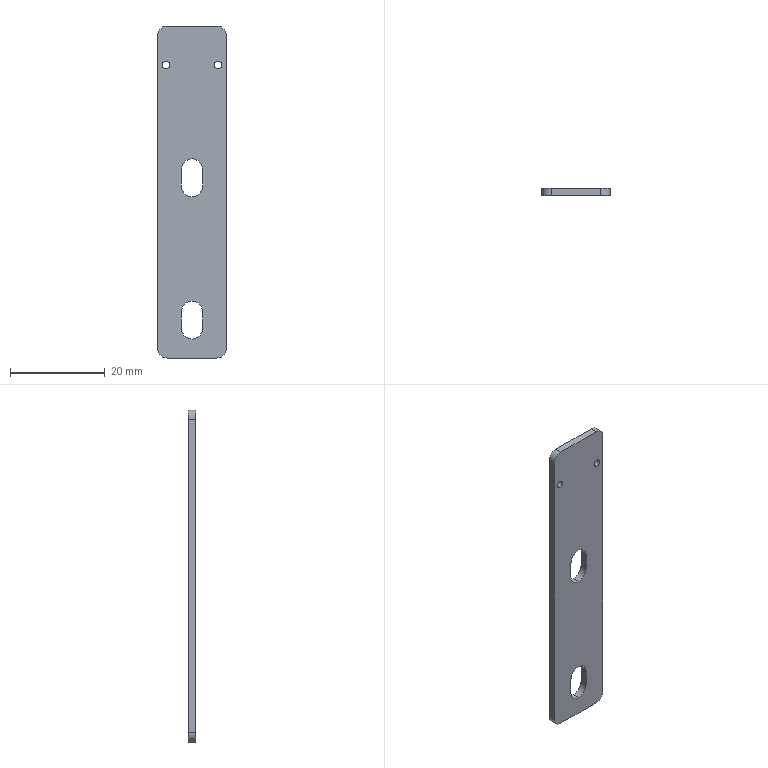Part | STEP file | through-beam photoelectric fixing plate | 1 solid | 24 faces | box 14.5 x 1.5 x 70 mm | volume 1416 mm3 | cylinder 14 | plane 10 | commonest cylinder face diameters 4.5 x6 1.6 x4 4 x4